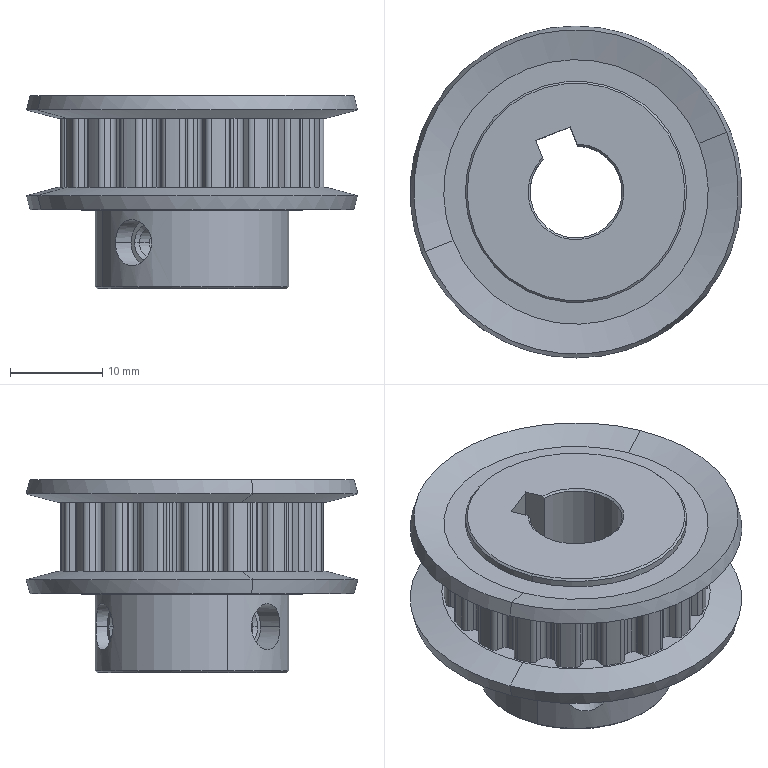Part | SolidWorks | features SplitBody 1 | 1 solid | 217 faces | box 36 x 36 x 21 mm | volume 9490 mm3 | cylinder 141 | plane 48 | cone 28 | commonest cylinder face diameters 1.22 x84 28.6 x19 25.8 x18 3.242 x4 5 x4 24 x4